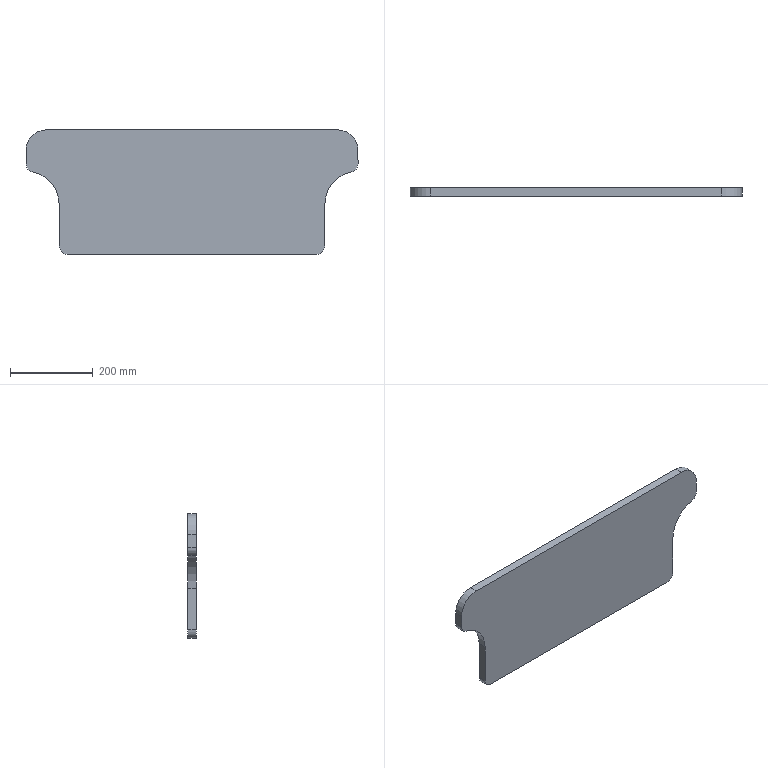Part | SolidWorks | features Fillet 2, Extrusion 1 | 1 solid | 16 faces | box 800 x 20 x 300 mm | volume 4187582 mm3 | plane 8 | cylinder 8 | commonest cylinder face diameters 40 x4 100 x2 160 x2
STEP:
#1=CARTESIAN_POINT('',(400.,-20.,100.));
#2=VERTEX_POINT('',#1);
#3=CARTESIAN_POINT('',(400.,-20.,67.98));
#4=VERTEX_POINT('',#3);
#5=CARTESIAN_POINT('',(400.,-20.,50.));
#6=DIRECTION('',(0.,0.,-1.));
#7=VECTOR('',#6,1000.);
#8=LINE('',#5,#7);
#9=EDGE_CURVE('',#2,#4,#8,.T.);
#10=ORIENTED_EDGE('',*,*,#9,.T.);
#11=CARTESIAN_POINT('',(400.,0.,67.98));
#12=VERTEX_POINT('',#11);
#13=CARTESIAN_POINT('',(400.,-20.,67.98));
#14=DIRECTION('',(0.,1.,0.));
#15=VECTOR('',#14,1000.);
#16=LINE('',#13,#15);
#17=EDGE_CURVE('',#4,#12,#16,.T.);
#18=ORIENTED_EDGE('',*,*,#17,.T.);
#19=CARTESIAN_POINT('',(400.,0.,100.));
#20=VERTEX_POINT('',#19);
#21=CARTESIAN_POINT('',(400.,0.,50.));
#22=DIRECTION('',(0.,0.,-1.));
#23=VECTOR('',#22,1000.);
#24=LINE('',#21,#23);
#25=EDGE_CURVE('',#20,#12,#24,.T.);
#26=ORIENTED_EDGE('',*,*,#25,.F.);
#27=CARTESIAN_POINT('',(400.,-20.,100.));
#28=DIRECTION('',(0.,-1.,0.));
#29=VECTOR('',#28,1000.);
#30=LINE('',#27,#29);
#31=EDGE_CURVE('',#20,#2,#30,.T.);
#32=ORIENTED_EDGE('',*,*,#31,.T.);
#33=EDGE_LOOP('',(#10,#18,#26,#32));
#34=FACE_OUTER_BOUND('',#33,.T.);
#35=CARTESIAN_POINT('',(400.,-20.,50.));
#36=DIRECTION('',(1.,0.,0.));
#37=DIRECTION('',(0.,0.,-1.));
#38=AXIS2_PLACEMENT_3D('',#35,#36,#37);
#39=PLANE('',#38);
#40=ADVANCED_FACE('',(#34),#39,.T.);
#41=CARTESIAN_POINT('',(-350.,-20.,150.));
#42=VERTEX_POINT('',#41);
#43=CARTESIAN_POINT('',(350.,-20.,150.));
#44=VERTEX_POINT('',#43);
#45=CARTESIAN_POINT('',(-400.,-20.,150.));
#46=DIRECTION('',(1.,0.,0.));
#47=VECTOR('',#46,1000.);
#48=LINE('',#45,#47);
#49=EDGE_CURVE('',#42,#44,#48,.T.);
#50=ORIENTED_EDGE('',*,*,#49,.T.);
#51=CARTESIAN_POINT('',(350.,0.,150.));
#52=VERTEX_POINT('',#51);
#53=CARTESIAN_POINT('',(350.,-20.,150.));
#54=DIRECTION('',(0.,1.,0.));
#55=VECTOR('',#54,1000.);
#56=LINE('',#53,#55);
#57=EDGE_CURVE('',#44,#52,#56,.T.);
#58=ORIENTED_EDGE('',*,*,#57,.T.);
#59=CARTESIAN_POINT('',(-350.,0.,150.));
#60=VERTEX_POINT('',#59);
#61=CARTESIAN_POINT('',(-400.,0.,150.));
#62=DIRECTION('',(1.,0.,0.));
#63=VECTOR('',#62,1000.);
#64=LINE('',#61,#63);
#65=EDGE_CURVE('',#60,#52,#64,.T.);
#66=ORIENTED_EDGE('',*,*,#65,.F.);
#67=CARTESIAN_POINT('',(-350.,-20.,150.));
#68=DIRECTION('',(0.,-1.,0.));
#69=VECTOR('',#68,1000.);
#70=LINE('',#67,#69);
#71=EDGE_CURVE('',#60,#42,#70,.T.);
#72=ORIENTED_EDGE('',*,*,#71,.T.);
#73=EDGE_LOOP('',(#50,#58,#66,#72));
#74=FACE_OUTER_BOUND('',#73,.T.);
#75=CARTESIAN_POINT('',(-400.,-20.,150.));
#76=DIRECTION('',(0.,0.,1.));
#77=DIRECTION('',(1.,0.,0.));
#78=AXIS2_PLACEMENT_3D('',#75,#76,#77);
#79=PLANE('',#78);
#80=ADVANCED_FACE('',(#74),#79,.T.);
#81=CARTESIAN_POINT('',(-400.,0.,67.98));
#82=VERTEX_POINT('',#81);
#83=CARTESIAN_POINT('',(-400.,0.,100.));
#84=VERTEX_POINT('',#83);
#85=CARTESIAN_POINT('',(-400.,0.,50.));
#86=DIRECTION('',(0.,0.,1.));
#87=VECTOR('',#86,1000.);
#88=LINE('',#85,#87);
#89=EDGE_CURVE('',#82,#84,#88,.T.);
#90=ORIENTED_EDGE('',*,*,#89,.F.);
#91=CARTESIAN_POINT('',(-400.,-20.,67.98));
#92=VERTEX_POINT('',#91);
#93=CARTESIAN_POINT('',(-400.,-20.,67.98));
#94=DIRECTION('',(0.,-1.,0.));
#95=VECTOR('',#94,1000.);
#96=LINE('',#93,#95);
#97=EDGE_CURVE('',#82,#92,#96,.T.);
#98=ORIENTED_EDGE('',*,*,#97,.T.);
#99=CARTESIAN_POINT('',(-400.,-20.,100.));
#100=VERTEX_POINT('',#99);
#101=CARTESIAN_POINT('',(-400.,-20.,50.));
#102=DIRECTION('',(0.,0.,1.));
#103=VECTOR('',#102,1000.);
#104=LINE('',#101,#103);
#105=EDGE_CURVE('',#92,#100,#104,.T.);
#106=ORIENTED_EDGE('',*,*,#105,.T.);
#107=CARTESIAN_POINT('',(-400.,-20.,100.));
#108=DIRECTION('',(0.,1.,0.));
#109=VECTOR('',#108,1000.);
#110=LINE('',#107,#109);
#111=EDGE_CURVE('',#100,#84,#110,.T.);
#112=ORIENTED_EDGE('',*,*,#111,.T.);
#113=EDGE_LOOP('',(#90,#98,#106,#112));
#114=FACE_OUTER_BOUND('',#113,.T.);
#115=CARTESIAN_POINT('',(-400.,-20.,50.));
#116=DIRECTION('',(-1.,0.,0.));
#117=DIRECTION('',(0.,0.,1.));
#118=AXIS2_PLACEMENT_3D('',#115,#116,#117);
#119=PLANE('',#118);
#120=ADVANCED_FACE('',(#114),#119,.T.);
#121=CARTESIAN_POINT('',(-320.,-20.,-30.));
#122=VERTEX_POINT('',#121);
#123=CARTESIAN_POINT('',(-384.,-20.,48.384));
#124=VERTEX_POINT('',#123);
#125=CARTESIAN_POINT('',(-400.,-20.,-30.));
#126=DIRECTION('',(0.,-1.,0.));
#127=DIRECTION('',(0.,0.,-1.));
#128=AXIS2_PLACEMENT_3D('',#125,#126,#127);
#129=CIRCLE('',#128,80.);
#130=EDGE_CURVE('',#122,#124,#129,.T.);
#131=ORIENTED_EDGE('',*,*,#130,.T.);
#132=CARTESIAN_POINT('',(-384.,0.,48.384));
#133=VERTEX_POINT('',#132);
#134=CARTESIAN_POINT('',(-384.,-20.,48.384));
#135=DIRECTION('',(0.,1.,0.));
#136=VECTOR('',#135,1000.);
#137=LINE('',#134,#136);
#138=EDGE_CURVE('',#124,#133,#137,.T.);
#139=ORIENTED_EDGE('',*,*,#138,.T.);
#140=CARTESIAN_POINT('',(-320.,0.,-30.));
#141=VERTEX_POINT('',#140);
#142=CARTESIAN_POINT('',(-400.,0.,-30.));
#143=DIRECTION('',(0.,-1.,0.));
#144=DIRECTION('',(0.,0.,-1.));
#145=AXIS2_PLACEMENT_3D('',#142,#143,#144);
#146=CIRCLE('',#145,80.);
#147=EDGE_CURVE('',#141,#133,#146,.T.);
#148=ORIENTED_EDGE('',*,*,#147,.F.);
#149=CARTESIAN_POINT('',(-320.,-20.,-30.));
#150=DIRECTION('',(0.,1.,0.));
#151=VECTOR('',#150,1000.);
#152=LINE('',#149,#151);
#153=EDGE_CURVE('',#122,#141,#152,.T.);
#154=ORIENTED_EDGE('',*,*,#153,.F.);
#155=EDGE_LOOP('',(#131,#139,#148,#154));
#156=FACE_OUTER_BOUND('',#155,.T.);
#157=CARTESIAN_POINT('',(-400.,-20.,-30.));
#158=DIRECTION('',(0.,1.,0.));
#159=DIRECTION('',(0.,0.,1.));
#160=AXIS2_PLACEMENT_3D('',#157,#158,#159);
#161=CYLINDRICAL_SURFACE('',#160,80.);
#162=ADVANCED_FACE('',(#156),#161,.F.);
#163=CARTESIAN_POINT('',(-320.,0.,-130.));
#164=VERTEX_POINT('',#163);
#165=CARTESIAN_POINT('',(-320.,0.,-150.));
#166=DIRECTION('',(0.,0.,1.));
#167=VECTOR('',#166,1000.);
#168=LINE('',#165,#167);
#169=EDGE_CURVE('',#164,#141,#168,.T.);
#170=ORIENTED_EDGE('',*,*,#169,.F.);
#171=CARTESIAN_POINT('',(-320.,-20.,-130.));
#172=VERTEX_POINT('',#171);
#173=CARTESIAN_POINT('',(-320.,-20.,-130.));
#174=DIRECTION('',(0.,-1.,0.));
#175=VECTOR('',#174,1000.);
#176=LINE('',#173,#175);
#177=EDGE_CURVE('',#164,#172,#176,.T.);
#178=ORIENTED_EDGE('',*,*,#177,.T.);
#179=CARTESIAN_POINT('',(-320.,-20.,-150.));
#180=DIRECTION('',(0.,0.,1.));
#181=VECTOR('',#180,1000.);
#182=LINE('',#179,#181);
#183=EDGE_CURVE('',#172,#122,#182,.T.);
#184=ORIENTED_EDGE('',*,*,#183,.T.);
#185=ORIENTED_EDGE('',*,*,#153,.T.);
#186=EDGE_LOOP('',(#170,#178,#184,#185));
#187=FACE_OUTER_BOUND('',#186,.T.);
#188=CARTESIAN_POINT('',(-320.,-20.,-150.));
#189=DIRECTION('',(-1.,0.,0.));
#190=DIRECTION('',(0.,0.,1.));
#191=AXIS2_PLACEMENT_3D('',#188,#189,#190);
#192=PLANE('',#191);
#193=ADVANCED_FACE('',(#187),#192,.T.);
#194=CARTESIAN_POINT('',(300.,-20.,-150.));
#195=VERTEX_POINT('',#194);
#196=CARTESIAN_POINT('',(-300.,-20.,-150.));
#197=VERTEX_POINT('',#196);
#198=CARTESIAN_POINT('',(-320.,-20.,-150.));
#199=DIRECTION('',(-1.,0.,0.));
#200=VECTOR('',#199,1000.);
#201=LINE('',#198,#200);
#202=EDGE_CURVE('',#195,#197,#201,.T.);
#203=ORIENTED_EDGE('',*,*,#202,.T.);
#204=CARTESIAN_POINT('',(-300.,0.,-150.));
#205=VERTEX_POINT('',#204);
#206=CARTESIAN_POINT('',(-300.,-20.,-150.));
#207=DIRECTION('',(0.,1.,0.));
#208=VECTOR('',#207,1000.);
#209=LINE('',#206,#208);
#210=EDGE_CURVE('',#197,#205,#209,.T.);
#211=ORIENTED_EDGE('',*,*,#210,.T.);
#212=CARTESIAN_POINT('',(300.,0.,-150.));
#213=VERTEX_POINT('',#212);
#214=CARTESIAN_POINT('',(-320.,0.,-150.));
#215=DIRECTION('',(-1.,0.,0.));
#216=VECTOR('',#215,1000.);
#217=LINE('',#214,#216);
#218=EDGE_CURVE('',#213,#205,#217,.T.);
#219=ORIENTED_EDGE('',*,*,#218,.F.);
#220=CARTESIAN_POINT('',(300.,-20.,-150.));
#221=DIRECTION('',(0.,-1.,0.));
#222=VECTOR('',#221,1000.);
#223=LINE('',#220,#222);
#224=EDGE_CURVE('',#213,#195,#223,.T.);
#225=ORIENTED_EDGE('',*,*,#224,.T.);
#226=EDGE_LOOP('',(#203,#211,#219,#225));
#227=FACE_OUTER_BOUND('',#226,.T.);
#228=CARTESIAN_POINT('',(-320.,-20.,-150.));
#229=DIRECTION('',(0.,0.,-1.));
#230=DIRECTION('',(-1.,0.,0.));
#231=AXIS2_PLACEMENT_3D('',#228,#229,#230);
#232=PLANE('',#231);
#233=ADVANCED_FACE('',(#227),#232,.T.);
#234=CARTESIAN_POINT('',(320.,-20.,-30.));
#235=VERTEX_POINT('',#234);
#236=CARTESIAN_POINT('',(320.,-20.,-130.));
#237=VERTEX_POINT('',#236);
#238=CARTESIAN_POINT('',(320.,-20.,-150.));
#239=DIRECTION('',(0.,0.,-1.));
#240=VECTOR('',#239,1000.);
#241=LINE('',#238,#240);
#242=EDGE_CURVE('',#235,#237,#241,.T.);
#243=ORIENTED_EDGE('',*,*,#242,.T.);
#244=CARTESIAN_POINT('',(320.,0.,-130.));
#245=VERTEX_POINT('',#244);
#246=CARTESIAN_POINT('',(320.,-20.,-130.));
#247=DIRECTION('',(0.,1.,0.));
#248=VECTOR('',#247,1000.);
#249=LINE('',#246,#248);
#250=EDGE_CURVE('',#237,#245,#249,.T.);
#251=ORIENTED_EDGE('',*,*,#250,.T.);
#252=CARTESIAN_POINT('',(320.,0.,-30.));
#253=VERTEX_POINT('',#252);
#254=CARTESIAN_POINT('',(320.,0.,-150.));
#255=DIRECTION('',(0.,0.,-1.));
#256=VECTOR('',#255,1000.);
#257=LINE('',#254,#256);
#258=EDGE_CURVE('',#253,#245,#257,.T.);
#259=ORIENTED_EDGE('',*,*,#258,.F.);
#260=CARTESIAN_POINT('',(320.,-20.,-30.));
#261=DIRECTION('',(0.,1.,0.));
#262=VECTOR('',#261,1000.);
#263=LINE('',#260,#262);
#264=EDGE_CURVE('',#235,#253,#263,.T.);
#265=ORIENTED_EDGE('',*,*,#264,.F.);
#266=EDGE_LOOP('',(#243,#251,#259,#265));
#267=FACE_OUTER_BOUND('',#266,.T.);
#268=CARTESIAN_POINT('',(320.,-20.,-150.));
#269=DIRECTION('',(1.,0.,0.));
#270=DIRECTION('',(0.,0.,-1.));
#271=AXIS2_PLACEMENT_3D('',#268,#269,#270);
#272=PLANE('',#271);
#273=ADVANCED_FACE('',(#267),#272,.T.);
#274=CARTESIAN_POINT('',(384.,0.,48.384));
#275=VERTEX_POINT('',#274);
#276=CARTESIAN_POINT('',(400.,0.,-30.));
#277=DIRECTION('',(0.,-1.,0.));
#278=DIRECTION('',(0.,0.,1.));
#279=AXIS2_PLACEMENT_3D('',#276,#277,#278);
#280=CIRCLE('',#279,80.);
#281=EDGE_CURVE('',#275,#253,#280,.T.);
#282=ORIENTED_EDGE('',*,*,#281,.F.);
#283=CARTESIAN_POINT('',(384.,-20.,48.384));
#284=VERTEX_POINT('',#283);
#285=CARTESIAN_POINT('',(384.,-20.,48.384));
#286=DIRECTION('',(0.,-1.,0.));
#287=VECTOR('',#286,1000.);
#288=LINE('',#285,#287);
#289=EDGE_CURVE('',#275,#284,#288,.T.);
#290=ORIENTED_EDGE('',*,*,#289,.T.);
#291=CARTESIAN_POINT('',(400.,-20.,-30.));
#292=DIRECTION('',(0.,-1.,0.));
#293=DIRECTION('',(0.,0.,1.));
#294=AXIS2_PLACEMENT_3D('',#291,#292,#293);
#295=CIRCLE('',#294,80.);
#296=EDGE_CURVE('',#284,#235,#295,.T.);
#297=ORIENTED_EDGE('',*,*,#296,.T.);
#298=ORIENTED_EDGE('',*,*,#264,.T.);
#299=EDGE_LOOP('',(#282,#290,#297,#298));
#300=FACE_OUTER_BOUND('',#299,.T.);
#301=CARTESIAN_POINT('',(400.,-20.,-30.));
#302=DIRECTION('',(0.,1.,0.));
#303=DIRECTION('',(0.,0.,1.));
#304=AXIS2_PLACEMENT_3D('',#301,#302,#303);
#305=CYLINDRICAL_SURFACE('',#304,80.);
#306=ADVANCED_FACE('',(#300),#305,.F.);
#307=ORIENTED_EDGE('',*,*,#296,.F.);
#308=CARTESIAN_POINT('',(380.,-20.,67.98));
#309=DIRECTION('',(0.,-1.,0.));
#310=DIRECTION('',(0.,0.,-1.));
#311=AXIS2_PLACEMENT_3D('',#308,#309,#310);
#312=CIRCLE('',#311,20.);
#313=EDGE_CURVE('',#284,#4,#312,.T.);
#314=ORIENTED_EDGE('',*,*,#313,.T.);
#315=ORIENTED_EDGE('',*,*,#9,.F.);
#316=CARTESIAN_POINT('',(350.,-20.,100.));
#317=DIRECTION('',(0.,-1.,0.));
#318=DIRECTION('',(0.,0.,-1.));
#319=AXIS2_PLACEMENT_3D('',#316,#317,#318);
#320=CIRCLE('',#319,50.);
#321=EDGE_CURVE('',#2,#44,#320,.T.);
#322=ORIENTED_EDGE('',*,*,#321,.T.);
#323=ORIENTED_EDGE('',*,*,#49,.F.);
#324=CARTESIAN_POINT('',(-350.,-20.,100.));
#325=DIRECTION('',(0.,-1.,0.));
#326=DIRECTION('',(0.,0.,-1.));
#327=AXIS2_PLACEMENT_3D('',#324,#325,#326);
#328=CIRCLE('',#327,50.);
#329=EDGE_CURVE('',#42,#100,#328,.T.);
#330=ORIENTED_EDGE('',*,*,#329,.T.);
#331=ORIENTED_EDGE('',*,*,#105,.F.);
#332=CARTESIAN_POINT('',(-380.,-20.,67.98));
#333=DIRECTION('',(0.,-1.,0.));
#334=DIRECTION('',(0.,0.,-1.));
#335=AXIS2_PLACEMENT_3D('',#332,#333,#334);
#336=CIRCLE('',#335,20.);
#337=EDGE_CURVE('',#92,#124,#336,.T.);
#338=ORIENTED_EDGE('',*,*,#337,.T.);
#339=ORIENTED_EDGE('',*,*,#130,.F.);
#340=ORIENTED_EDGE('',*,*,#183,.F.);
#341=CARTESIAN_POINT('',(-300.,-20.,-130.));
#342=DIRECTION('',(0.,-1.,0.));
#343=DIRECTION('',(0.,0.,-1.));
#344=AXIS2_PLACEMENT_3D('',#341,#342,#343);
#345=CIRCLE('',#344,20.);
#346=EDGE_CURVE('',#172,#197,#345,.T.);
#347=ORIENTED_EDGE('',*,*,#346,.T.);
#348=ORIENTED_EDGE('',*,*,#202,.F.);
#349=CARTESIAN_POINT('',(300.,-20.,-130.));
#350=DIRECTION('',(0.,-1.,0.));
#351=DIRECTION('',(0.,0.,-1.));
#352=AXIS2_PLACEMENT_3D('',#349,#350,#351);
#353=CIRCLE('',#352,20.);
#354=EDGE_CURVE('',#195,#237,#353,.T.);
#355=ORIENTED_EDGE('',*,*,#354,.T.);
#356=ORIENTED_EDGE('',*,*,#242,.F.);
#357=EDGE_LOOP('',(#307,#314,#315,#322,#323,#330,#331,#338,#339,#340,#347,#348,#355,#356));
#358=FACE_OUTER_BOUND('',#357,.T.);
#359=CARTESIAN_POINT('',(-400.,-20.,-30.));
#360=DIRECTION('',(0.,-1.,0.));
#361=DIRECTION('',(0.,0.,-1.));
#362=AXIS2_PLACEMENT_3D('',#359,#360,#361);
#363=PLANE('',#362);
#364=ADVANCED_FACE('',(#358),#363,.T.);
#365=ORIENTED_EDGE('',*,*,#25,.T.);
#366=CARTESIAN_POINT('',(380.,0.,67.98));
#367=DIRECTION('',(0.,1.,0.));
#368=DIRECTION('',(0.,0.,-1.));
#369=AXIS2_PLACEMENT_3D('',#366,#367,#368);
#370=CIRCLE('',#369,20.);
#371=EDGE_CURVE('',#12,#275,#370,.T.);
#372=ORIENTED_EDGE('',*,*,#371,.T.);
#373=ORIENTED_EDGE('',*,*,#281,.T.);
#374=ORIENTED_EDGE('',*,*,#258,.T.);
#375=CARTESIAN_POINT('',(300.,0.,-130.));
#376=DIRECTION('',(0.,1.,0.));
#377=DIRECTION('',(0.,0.,-1.));
#378=AXIS2_PLACEMENT_3D('',#375,#376,#377);
#379=CIRCLE('',#378,20.);
#380=EDGE_CURVE('',#245,#213,#379,.T.);
#381=ORIENTED_EDGE('',*,*,#380,.T.);
#382=ORIENTED_EDGE('',*,*,#218,.T.);
#383=CARTESIAN_POINT('',(-300.,0.,-130.));
#384=DIRECTION('',(0.,1.,0.));
#385=DIRECTION('',(0.,0.,-1.));
#386=AXIS2_PLACEMENT_3D('',#383,#384,#385);
#387=CIRCLE('',#386,20.);
#388=EDGE_CURVE('',#205,#164,#387,.T.);
#389=ORIENTED_EDGE('',*,*,#388,.T.);
#390=ORIENTED_EDGE('',*,*,#169,.T.);
#391=ORIENTED_EDGE('',*,*,#147,.T.);
#392=CARTESIAN_POINT('',(-380.,0.,67.98));
#393=DIRECTION('',(0.,1.,0.));
#394=DIRECTION('',(0.,0.,-1.));
#395=AXIS2_PLACEMENT_3D('',#392,#393,#394);
#396=CIRCLE('',#395,20.);
#397=EDGE_CURVE('',#133,#82,#396,.T.);
#398=ORIENTED_EDGE('',*,*,#397,.T.);
#399=ORIENTED_EDGE('',*,*,#89,.T.);
#400=CARTESIAN_POINT('',(-350.,0.,100.));
#401=DIRECTION('',(0.,1.,0.));
#402=DIRECTION('',(0.,0.,-1.));
#403=AXIS2_PLACEMENT_3D('',#400,#401,#402);
#404=CIRCLE('',#403,50.);
#405=EDGE_CURVE('',#84,#60,#404,.T.);
#406=ORIENTED_EDGE('',*,*,#405,.T.);
#407=ORIENTED_EDGE('',*,*,#65,.T.);
#408=CARTESIAN_POINT('',(350.,0.,100.));
#409=DIRECTION('',(0.,1.,0.));
#410=DIRECTION('',(0.,0.,-1.));
#411=AXIS2_PLACEMENT_3D('',#408,#409,#410);
#412=CIRCLE('',#411,50.);
#413=EDGE_CURVE('',#52,#20,#412,.T.);
#414=ORIENTED_EDGE('',*,*,#413,.T.);
#415=EDGE_LOOP('',(#365,#372,#373,#374,#381,#382,#389,#390,#391,#398,#399,#406,#407,#414));
#416=FACE_OUTER_BOUND('',#415,.T.);
#417=CARTESIAN_POINT('',(-400.,0.,-30.));
#418=DIRECTION('',(0.,-1.,0.));
#419=DIRECTION('',(0.,0.,-1.));
#420=AXIS2_PLACEMENT_3D('',#417,#418,#419);
#421=PLANE('',#420);
#422=ADVANCED_FACE('',(#416),#421,.F.);
#423=ORIENTED_EDGE('',*,*,#321,.F.);
#424=ORIENTED_EDGE('',*,*,#31,.F.);
#425=ORIENTED_EDGE('',*,*,#413,.F.);
#426=ORIENTED_EDGE('',*,*,#57,.F.);
#427=EDGE_LOOP('',(#423,#424,#425,#426));
#428=FACE_OUTER_BOUND('',#427,.T.);
#429=CARTESIAN_POINT('',(350.,-20.,100.));
#430=DIRECTION('',(0.,1.,0.));
#431=DIRECTION('',(0.,0.,1.));
#432=AXIS2_PLACEMENT_3D('',#429,#430,#431);
#433=CYLINDRICAL_SURFACE('',#432,50.);
#434=ADVANCED_FACE('',(#428),#433,.T.);
#435=ORIENTED_EDGE('',*,*,#329,.F.);
#436=ORIENTED_EDGE('',*,*,#71,.F.);
#437=ORIENTED_EDGE('',*,*,#405,.F.);
#438=ORIENTED_EDGE('',*,*,#111,.F.);
#439=EDGE_LOOP('',(#435,#436,#437,#438));
#440=FACE_OUTER_BOUND('',#439,.T.);
#441=CARTESIAN_POINT('',(-350.,-20.,100.));
#442=DIRECTION('',(0.,1.,0.));
#443=DIRECTION('',(0.,0.,1.));
#444=AXIS2_PLACEMENT_3D('',#441,#442,#443);
#445=CYLINDRICAL_SURFACE('',#444,50.);
#446=ADVANCED_FACE('',(#440),#445,.T.);
#447=ORIENTED_EDGE('',*,*,#313,.F.);
#448=ORIENTED_EDGE('',*,*,#289,.F.);
#449=ORIENTED_EDGE('',*,*,#371,.F.);
#450=ORIENTED_EDGE('',*,*,#17,.F.);
#451=EDGE_LOOP('',(#447,#448,#449,#450));
#452=FACE_OUTER_BOUND('',#451,.T.);
#453=CARTESIAN_POINT('',(380.,-20.,67.98));
#454=DIRECTION('',(0.,1.,0.));
#455=DIRECTION('',(0.,0.,1.));
#456=AXIS2_PLACEMENT_3D('',#453,#454,#455);
#457=CYLINDRICAL_SURFACE('',#456,20.);
#458=ADVANCED_FACE('',(#452),#457,.T.);
#459=ORIENTED_EDGE('',*,*,#337,.F.);
#460=ORIENTED_EDGE('',*,*,#97,.F.);
#461=ORIENTED_EDGE('',*,*,#397,.F.);
#462=ORIENTED_EDGE('',*,*,#138,.F.);
#463=EDGE_LOOP('',(#459,#460,#461,#462));
#464=FACE_OUTER_BOUND('',#463,.T.);
#465=CARTESIAN_POINT('',(-380.,-20.,67.98));
#466=DIRECTION('',(0.,1.,0.));
#467=DIRECTION('',(0.,0.,1.));
#468=AXIS2_PLACEMENT_3D('',#465,#466,#467);
#469=CYLINDRICAL_SURFACE('',#468,20.);
#470=ADVANCED_FACE('',(#464),#469,.T.);
#471=ORIENTED_EDGE('',*,*,#346,.F.);
#472=ORIENTED_EDGE('',*,*,#177,.F.);
#473=ORIENTED_EDGE('',*,*,#388,.F.);
#474=ORIENTED_EDGE('',*,*,#210,.F.);
#475=EDGE_LOOP('',(#471,#472,#473,#474));
#476=FACE_OUTER_BOUND('',#475,.T.);
#477=CARTESIAN_POINT('',(-300.,-20.,-130.));
#478=DIRECTION('',(0.,1.,0.));
#479=DIRECTION('',(0.,0.,1.));
#480=AXIS2_PLACEMENT_3D('',#477,#478,#479);
#481=CYLINDRICAL_SURFACE('',#480,20.);
#482=ADVANCED_FACE('',(#476),#481,.T.);
#483=ORIENTED_EDGE('',*,*,#354,.F.);
#484=ORIENTED_EDGE('',*,*,#224,.F.);
#485=ORIENTED_EDGE('',*,*,#380,.F.);
#486=ORIENTED_EDGE('',*,*,#250,.F.);
#487=EDGE_LOOP('',(#483,#484,#485,#486));
#488=FACE_OUTER_BOUND('',#487,.T.);
#489=CARTESIAN_POINT('',(300.,-20.,-130.));
#490=DIRECTION('',(0.,1.,0.));
#491=DIRECTION('',(0.,0.,1.));
#492=AXIS2_PLACEMENT_3D('',#489,#490,#491);
#493=CYLINDRICAL_SURFACE('',#492,20.);
#494=ADVANCED_FACE('',(#488),#493,.T.);
#495=CLOSED_SHELL('',(#40,#80,#120,#162,#193,#233,#273,#306,#364,#422,#434,#446,#458,#470,#482,#494));
#496=MANIFOLD_SOLID_BREP('',#495);
#497=CARTESIAN_POINT('',(0.,0.,0.));
#498=DIRECTION('',(0.,0.,1.));
#499=DIRECTION('',(1.,0.,0.));
#500=AXIS2_PLACEMENT_3D('',#497,#498,#499);
#501=(LENGTH_UNIT()NAMED_UNIT(*)SI_UNIT(.MILLI.,.METRE.));
#502=UNCERTAINTY_MEASURE_WITH_UNIT(LENGTH_MEASURE(0.00001),#501,'','');
#503=(NAMED_UNIT(*)PLANE_ANGLE_UNIT()SI_UNIT($,.RADIAN.));
#504=(NAMED_UNIT(*)SI_UNIT($,.STERADIAN.)SOLID_ANGLE_UNIT());
#505=(GEOMETRIC_REPRESENTATION_CONTEXT(3)GLOBAL_UNCERTAINTY_ASSIGNED_CONTEXT((#502))GLOBAL_UNIT_ASSIGNED_CONTEXT((#501,#503,#504))REPRESENTATION_CONTEXT('',''));
#506=ADVANCED_BREP_SHAPE_REPRESENTATION('',(#496,#500),#505);